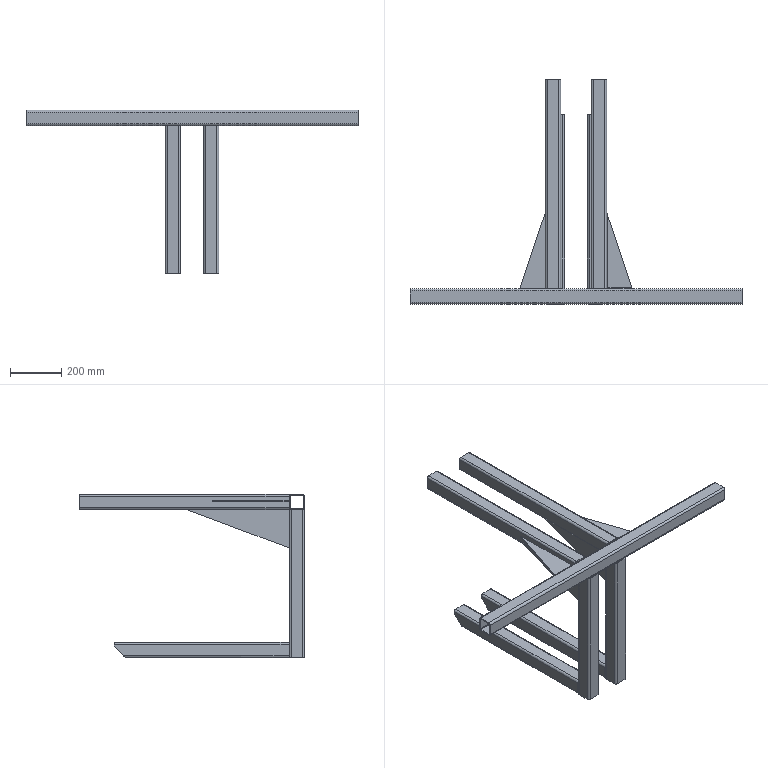Part | SolidWorks | features Gusset 4, WeldMemberFeat 3, WeldCornerFeat 2, ICE 1, WeldBeadFeat 1, WeldmentFeature 1 | 13 solids | 162 faces | box 1300 x 880 x 640 mm | volume 6179096 mm3 | plane 106 | cylinder 56 | commonest cylinder face diameters 6 x28 16 x28